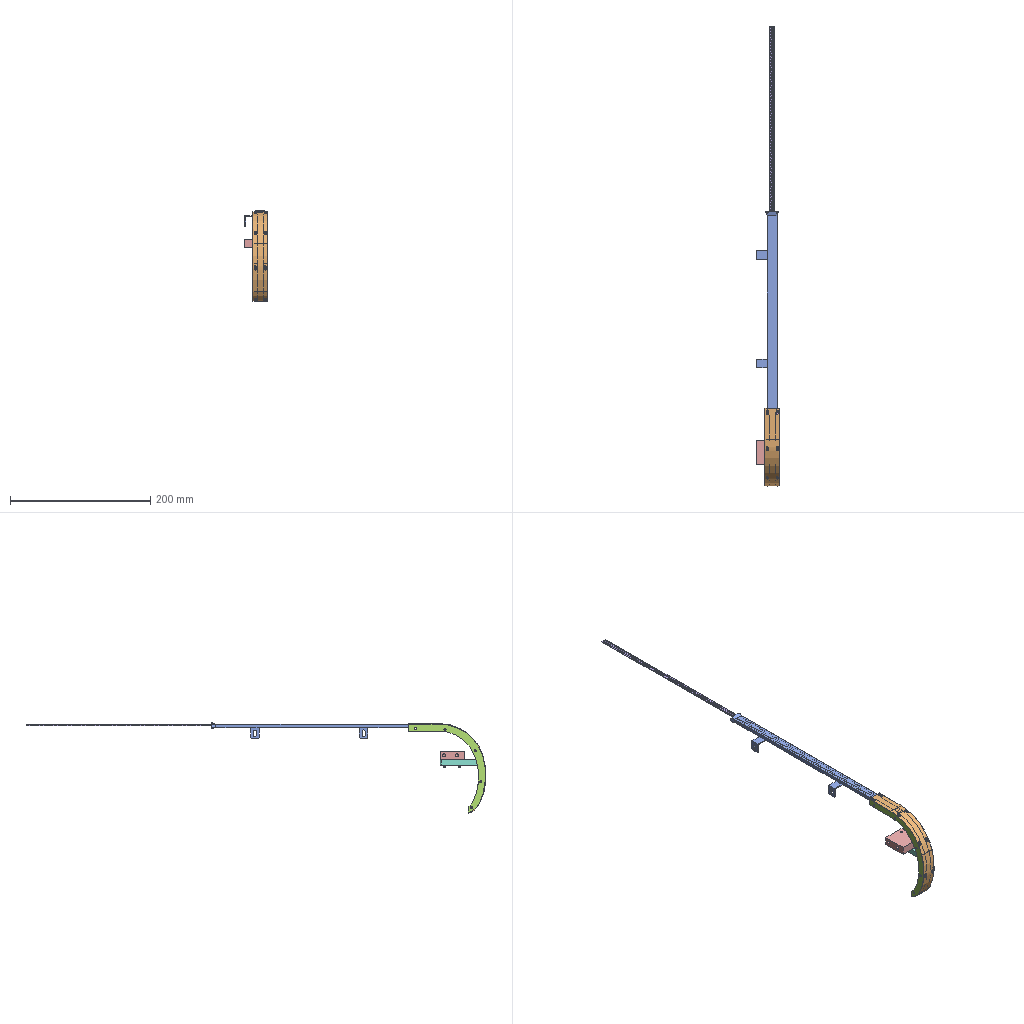Assembly | SolidWorks | 8 different items | 9 placed | box 32 x 656 x 129 mm
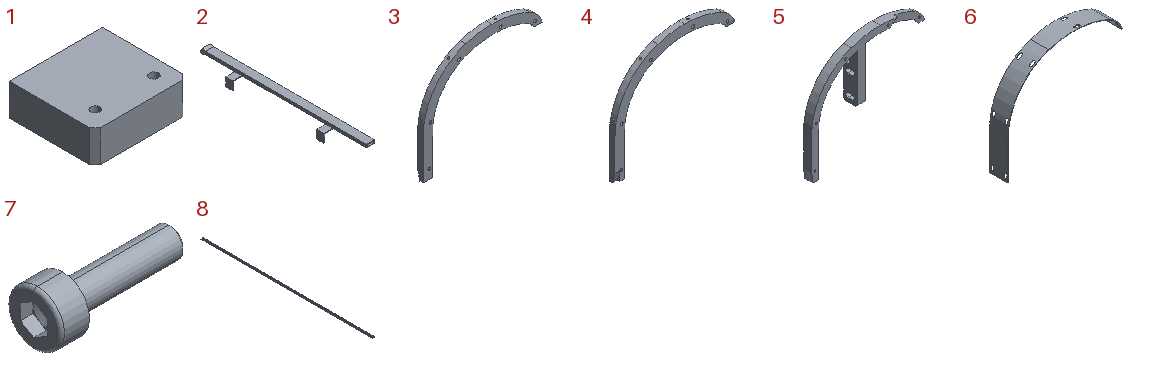Parts list (item | quantity | size | volume | features):
1 | x1 | 35 x 32.2 x 12 mm | 12915 mm3 | features 3DProfileFeature 2, HoleWzd 2, Chamfer 1, Extrusion 1
2 | x1 | 30.899 x 280.673 x 21.992 mm | 10987 mm3 | features ICE 5, Fillet 3, Chamfer 1, Extrusion 1, LPattern 1, MirrorPattern 1
3 | x1 | 126.964 x 6 x 110 mm | 11727 mm3 | features ICE 3, Cut 2, 3DProfileFeature 1, Chamfer 1, CurvePattern 1, Extrusion 1, HoleWzd 1
4 | x1 | 126.964 x 6 x 110 mm | 11727 mm3 | features ICE 3, Cut 2, Chamfer 1, CurvePattern 1, Extrusion 1, HoleWzd 1
5 | x1 | 121.296 x 14.4 x 107 mm | 14940 mm3 | features ICE 8, Chamfer 3, HoleWzd 2, Extrusion 1
6 | x1 | 127.94 x 20.4 x 110.5 mm | 2142 mm3 | features ICE 6, CurvePattern 1, Extrusion 1
7 | x2 | 7.6 x 3 x 3 mm | 21.652 mm3 | features Fillet 2, RevCut 2, Boss 1, Chamfer 1, Cut 1, Extrusion 1, LPattern 1
8 | x1 | 8 x 600 x 1.5 mm | 1218 mm3 | features ICE 4, LPattern 4, Extrusion 1
Mates (type | each side: item.copy, entity, surface, feature):
Coincident | 2.1 face plane Boss-Extrude1 | 8.1 face plane Boss-Extrude1 | 2 times
Concentric | 1.1 face cylinder M4 Tapped Hole1 | 7.1 face cylinder BaseBody
Concentric | 1.1 face cylinder M4 Tapped Hole1 | 7.2 face cylinder BaseBody
DistanceDim | 8.1 face plane Boss-Extrude1 | 2.1 face plane Boss-Extrude1
Coincident | 2.1 face plane Boss-Extrude1 | 3.1 face plane Boss-Extrude1 | 2 times
Coincident | 3.1 face plane Boss-Extrude1 | 4.1 face plane Boss-Extrude1
Coincident | 2.1 face plane Boss-Extrude1 | 4.1 face plane Boss-Extrude1
Coincident | 4.1 face plane Boss-Extrude1 | 5.1 face plane Boss-Extrude1
Coincident | 4.1 face plane Boss-Extrude1 | 5.1 face plane Cut-Extrude4
Coincident | 3.1 face plane Cut-Extrude2 | 5.1 face plane Cut-Extrude2
Coincident | 1.1 face plane Boss-Extrude1 | 5.1 face plane Boss-Extrude2 | 2 times
Coincident | 1.1 face plane Boss-Extrude1 | 5.1 face plane Boss-Extrude1
Coincident | 4.1 face plane Boss-Extrude1 | 6.1 face plane Boss-Extrude2 | 3 times
Coincident | 1.1 face plane Boss-Extrude1 | 2.1 face plane LPattern1